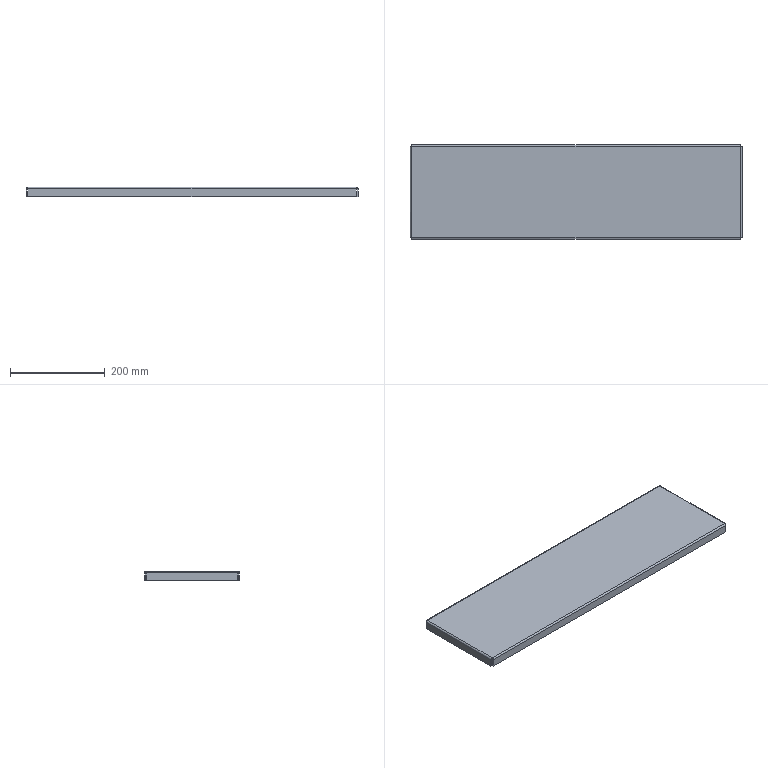Part | STEP file | PN_0008 top 304 stair tread_Default<As Machined> | 1 solid | 38 faces | box 700 x 200 x 20 mm | volume 506035 mm3 | plane 22 | spline 8 | cylinder 8 | commonest cylinder face diameters 0.6 x4 6.6 x4